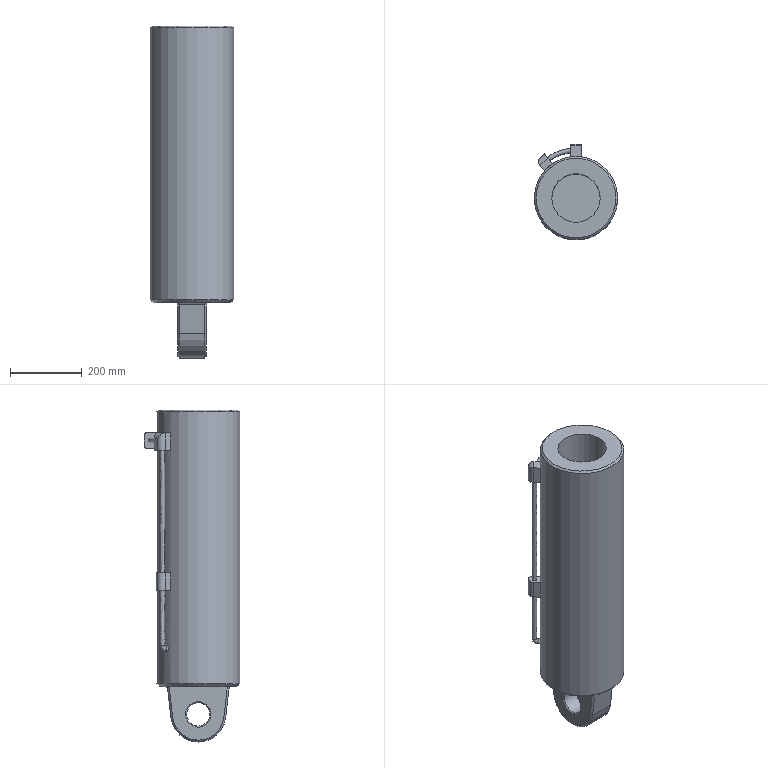Part | NX | features 平衡千斤顶缸 2 | 1 solid | 52 faces | box 232.246 x 266.383 x 924.565 mm | volume 24015479 mm3 | plane 25 | cylinder 12 | cone 10 | spline 5 | commonest cylinder face diameters 10 x4 30 x4 65 x1 135 x1 153.5 x1 232.246 x1